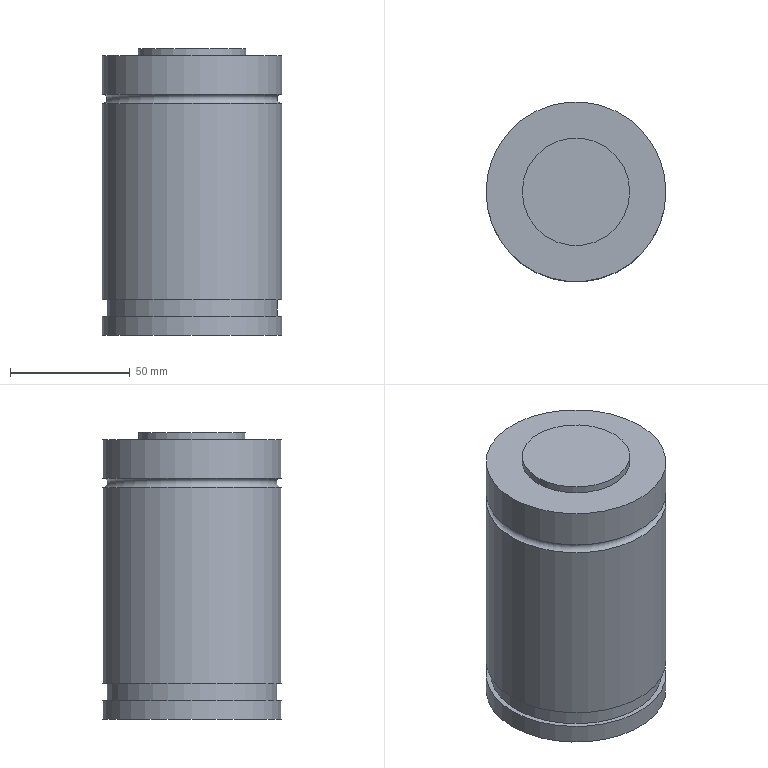Part | NX | features MAIN_BODY 2 | 1 solid | 11 faces | box 75.2 x 75.2 x 120 mm | volume 519752 mm3 | cylinder 5 | plane 5 | torus 1 | commonest cylinder face diameters 75.2 x3 45 x1 71.2 x1
STEP:
#1=CARTESIAN_POINT('',(-612.35,-310.,110.));
#2=VERTEX_POINT('',#1);
#3=CARTESIAN_POINT('',(-574.75,-310.,110.));
#4=DIRECTION('',(0.,0.,1.));
#5=DIRECTION('',(-1.,0.,0.));
#6=AXIS2_PLACEMENT_3D('',#3,#4,#5);
#7=CIRCLE('',#6,37.6);
#8=EDGE_CURVE('',#2,#2,#7,.F.);
#9=ORIENTED_EDGE('',*,*,#8,.F.);
#10=EDGE_LOOP('',(#9));
#11=FACE_BOUND('',#10,.T.);
#12=CARTESIAN_POINT('',(-612.35,-310.,192.));
#13=VERTEX_POINT('',#12);
#14=CARTESIAN_POINT('',(-574.75,-310.,192.));
#15=DIRECTION('',(0.,0.,1.));
#16=DIRECTION('',(-1.,0.,0.));
#17=AXIS2_PLACEMENT_3D('',#14,#15,#16);
#18=CIRCLE('',#17,37.6);
#19=EDGE_CURVE('',#13,#13,#18,.T.);
#20=ORIENTED_EDGE('',*,*,#19,.F.);
#21=EDGE_LOOP('',(#20));
#22=FACE_BOUND('',#21,.T.);
#23=CARTESIAN_POINT('',(-574.75,-310.,212.));
#24=DIRECTION('',(0.,0.,-1.));
#25=DIRECTION('',(-1.,0.,0.));
#26=AXIS2_PLACEMENT_3D('',#23,#24,#25);
#27=CYLINDRICAL_SURFACE('',#26,37.6);
#28=ADVANCED_FACE('',(#11,#22),#27,.T.);
#29=CARTESIAN_POINT('',(-537.15,-310.,212.));
#30=VERTEX_POINT('',#29);
#31=CARTESIAN_POINT('',(-574.75,-310.,212.));
#32=DIRECTION('',(0.,0.,-1.));
#33=DIRECTION('',(1.,0.,0.));
#34=AXIS2_PLACEMENT_3D('',#31,#32,#33);
#35=CIRCLE('',#34,37.6);
#36=EDGE_CURVE('',#30,#30,#35,.T.);
#37=ORIENTED_EDGE('',*,*,#36,.F.);
#38=EDGE_LOOP('',(#37));
#39=FACE_BOUND('',#38,.T.);
#40=CARTESIAN_POINT('',(-552.25,-310.,212.));
#41=VERTEX_POINT('',#40);
#42=CARTESIAN_POINT('',(-574.75,-310.,212.));
#43=DIRECTION('',(0.,0.,-1.));
#44=DIRECTION('',(1.,0.,0.));
#45=AXIS2_PLACEMENT_3D('',#42,#43,#44);
#46=CIRCLE('',#45,22.5);
#47=EDGE_CURVE('',#41,#41,#46,.T.);
#48=ORIENTED_EDGE('',*,*,#47,.T.);
#49=EDGE_LOOP('',(#48));
#50=FACE_BOUND('',#49,.T.);
#51=CARTESIAN_POINT('',(-574.75,-310.,212.));
#52=DIRECTION('',(0.,0.,1.));
#53=DIRECTION('',(1.,0.,0.));
#54=AXIS2_PLACEMENT_3D('',#51,#52,#53);
#55=PLANE('',#54);
#56=ADVANCED_FACE('',(#39,#50),#55,.T.);
#57=CARTESIAN_POINT('',(-612.35,-310.,196.));
#58=VERTEX_POINT('',#57);
#59=CARTESIAN_POINT('',(-574.75,-310.,196.));
#60=DIRECTION('',(0.,0.,1.));
#61=DIRECTION('',(-1.,0.,0.));
#62=AXIS2_PLACEMENT_3D('',#59,#60,#61);
#63=CIRCLE('',#62,37.6);
#64=EDGE_CURVE('',#58,#58,#63,.F.);
#65=ORIENTED_EDGE('',*,*,#64,.F.);
#66=EDGE_LOOP('',(#65));
#67=FACE_BOUND('',#66,.T.);
#68=ORIENTED_EDGE('',*,*,#36,.T.);
#69=EDGE_LOOP('',(#68));
#70=FACE_BOUND('',#69,.T.);
#71=CARTESIAN_POINT('',(-574.75,-310.,212.));
#72=DIRECTION('',(0.,0.,-1.));
#73=DIRECTION('',(-1.,0.,0.));
#74=AXIS2_PLACEMENT_3D('',#71,#72,#73);
#75=CYLINDRICAL_SURFACE('',#74,37.6);
#76=ADVANCED_FACE('',(#67,#70),#75,.T.);
#77=CARTESIAN_POINT('',(-552.25,-310.,215.));
#78=VERTEX_POINT('',#77);
#79=CARTESIAN_POINT('',(-574.75,-310.,215.));
#80=DIRECTION('',(0.,0.,-1.));
#81=DIRECTION('',(1.,0.,0.));
#82=AXIS2_PLACEMENT_3D('',#79,#80,#81);
#83=CIRCLE('',#82,22.5);
#84=EDGE_CURVE('',#78,#78,#83,.T.);
#85=ORIENTED_EDGE('',*,*,#84,.T.);
#86=EDGE_LOOP('',(#85));
#87=FACE_BOUND('',#86,.T.);
#88=ORIENTED_EDGE('',*,*,#47,.F.);
#89=EDGE_LOOP('',(#88));
#90=FACE_BOUND('',#89,.T.);
#91=CARTESIAN_POINT('',(-574.75,-310.,215.));
#92=DIRECTION('',(0.,0.,-1.));
#93=DIRECTION('',(-1.,0.,0.));
#94=AXIS2_PLACEMENT_3D('',#91,#92,#93);
#95=CYLINDRICAL_SURFACE('',#94,22.5);
#96=ADVANCED_FACE('',(#87,#90),#95,.T.);
#97=ORIENTED_EDGE('',*,*,#84,.F.);
#98=EDGE_LOOP('',(#97));
#99=FACE_BOUND('',#98,.T.);
#100=CARTESIAN_POINT('',(-574.75,-310.,215.));
#101=DIRECTION('',(0.,0.,1.));
#102=DIRECTION('',(1.,0.,0.));
#103=AXIS2_PLACEMENT_3D('',#100,#101,#102);
#104=PLANE('',#103);
#105=ADVANCED_FACE('',(#99),#104,.T.);
#106=ORIENTED_EDGE('',*,*,#64,.T.);
#107=EDGE_LOOP('',(#106));
#108=FACE_BOUND('',#107,.T.);
#109=ORIENTED_EDGE('',*,*,#19,.T.);
#110=EDGE_LOOP('',(#109));
#111=FACE_BOUND('',#110,.T.);
#112=CARTESIAN_POINT('',(-574.75,-310.,194.));
#113=DIRECTION('',(0.,0.,-1.));
#114=DIRECTION('',(-1.,0.,0.));
#115=AXIS2_PLACEMENT_3D('',#112,#113,#114);
#116=TOROIDAL_SURFACE('',#115,37.6,2.);
#117=ADVANCED_FACE('',(#108,#111),#116,.F.);
#118=CARTESIAN_POINT('',(-539.15,-310.,110.));
#119=VERTEX_POINT('',#118);
#120=CARTESIAN_POINT('',(-574.75,-310.,110.));
#121=DIRECTION('',(0.,0.,-1.));
#122=DIRECTION('',(1.,0.,0.));
#123=AXIS2_PLACEMENT_3D('',#120,#121,#122);
#124=CIRCLE('',#123,35.6);
#125=EDGE_CURVE('',#119,#119,#124,.T.);
#126=ORIENTED_EDGE('',*,*,#125,.F.);
#127=EDGE_LOOP('',(#126));
#128=FACE_BOUND('',#127,.T.);
#129=ORIENTED_EDGE('',*,*,#8,.T.);
#130=EDGE_LOOP('',(#129));
#131=FACE_BOUND('',#130,.T.);
#132=CARTESIAN_POINT('',(-574.75,-310.,110.));
#133=DIRECTION('',(0.,0.,-1.));
#134=DIRECTION('',(-1.,0.,0.));
#135=AXIS2_PLACEMENT_3D('',#132,#133,#134);
#136=PLANE('',#135);
#137=ADVANCED_FACE('',(#128,#131),#136,.T.);
#138=CARTESIAN_POINT('',(-539.15,-310.,103.));
#139=VERTEX_POINT('',#138);
#140=CARTESIAN_POINT('',(-574.75,-310.,103.));
#141=DIRECTION('',(0.,0.,-1.));
#142=DIRECTION('',(1.,0.,0.));
#143=AXIS2_PLACEMENT_3D('',#140,#141,#142);
#144=CIRCLE('',#143,35.6);
#145=EDGE_CURVE('',#139,#139,#144,.T.);
#146=ORIENTED_EDGE('',*,*,#145,.T.);
#147=EDGE_LOOP('',(#146));
#148=FACE_BOUND('',#147,.T.);
#149=CARTESIAN_POINT('',(-612.35,-310.,103.));
#150=VERTEX_POINT('',#149);
#151=CARTESIAN_POINT('',(-574.75,-310.,103.));
#152=DIRECTION('',(0.,0.,1.));
#153=DIRECTION('',(-1.,0.,0.));
#154=AXIS2_PLACEMENT_3D('',#151,#152,#153);
#155=CIRCLE('',#154,37.6);
#156=EDGE_CURVE('',#150,#150,#155,.T.);
#157=ORIENTED_EDGE('',*,*,#156,.T.);
#158=EDGE_LOOP('',(#157));
#159=FACE_BOUND('',#158,.T.);
#160=CARTESIAN_POINT('',(-574.75,-310.,103.));
#161=DIRECTION('',(0.,0.,-1.));
#162=DIRECTION('',(-1.,0.,0.));
#163=AXIS2_PLACEMENT_3D('',#160,#161,#162);
#164=PLANE('',#163);
#165=ADVANCED_FACE('',(#148,#159),#164,.F.);
#166=ORIENTED_EDGE('',*,*,#125,.T.);
#167=EDGE_LOOP('',(#166));
#168=FACE_BOUND('',#167,.T.);
#169=ORIENTED_EDGE('',*,*,#145,.F.);
#170=EDGE_LOOP('',(#169));
#171=FACE_BOUND('',#170,.T.);
#172=CARTESIAN_POINT('',(-574.75,-310.,103.));
#173=DIRECTION('',(0.,0.,1.));
#174=DIRECTION('',(1.,0.,0.));
#175=AXIS2_PLACEMENT_3D('',#172,#173,#174);
#176=CYLINDRICAL_SURFACE('',#175,35.6);
#177=ADVANCED_FACE('',(#168,#171),#176,.T.);
#178=CARTESIAN_POINT('',(-537.15,-310.,95.));
#179=VERTEX_POINT('',#178);
#180=CARTESIAN_POINT('',(-574.75,-310.,95.));
#181=DIRECTION('',(0.,0.,-1.));
#182=DIRECTION('',(1.,0.,0.));
#183=AXIS2_PLACEMENT_3D('',#180,#181,#182);
#184=CIRCLE('',#183,37.6);
#185=EDGE_CURVE('',#179,#179,#184,.T.);
#186=ORIENTED_EDGE('',*,*,#185,.T.);
#187=EDGE_LOOP('',(#186));
#188=FACE_BOUND('',#187,.T.);
#189=CARTESIAN_POINT('',(-574.75,-310.,95.));
#190=DIRECTION('',(0.,0.,1.));
#191=DIRECTION('',(1.,0.,0.));
#192=AXIS2_PLACEMENT_3D('',#189,#190,#191);
#193=PLANE('',#192);
#194=ADVANCED_FACE('',(#188),#193,.F.);
#195=ORIENTED_EDGE('',*,*,#156,.F.);
#196=EDGE_LOOP('',(#195));
#197=FACE_BOUND('',#196,.T.);
#198=ORIENTED_EDGE('',*,*,#185,.F.);
#199=EDGE_LOOP('',(#198));
#200=FACE_BOUND('',#199,.T.);
#201=CARTESIAN_POINT('',(-574.75,-310.,212.));
#202=DIRECTION('',(0.,0.,-1.));
#203=DIRECTION('',(-1.,0.,0.));
#204=AXIS2_PLACEMENT_3D('',#201,#202,#203);
#205=CYLINDRICAL_SURFACE('',#204,37.6);
#206=ADVANCED_FACE('',(#197,#200),#205,.T.);
#207=CLOSED_SHELL('',(#28,#56,#76,#96,#105,#117,#137,#165,#177,#194,#206));
#208=MANIFOLD_SOLID_BREP('',#207);
#209=(LENGTH_UNIT()NAMED_UNIT(*)SI_UNIT(.MILLI.,.METRE.));
#210=UNCERTAINTY_MEASURE_WITH_UNIT(LENGTH_MEASURE(0.00001),#209,'','');
#211=(NAMED_UNIT(*)PLANE_ANGLE_UNIT()SI_UNIT($,.RADIAN.));
#212=(NAMED_UNIT(*)SI_UNIT($,.STERADIAN.)SOLID_ANGLE_UNIT());
#213=(GEOMETRIC_REPRESENTATION_CONTEXT(3)GLOBAL_UNCERTAINTY_ASSIGNED_CONTEXT((#210))GLOBAL_UNIT_ASSIGNED_CONTEXT((#209,#211,#212))REPRESENTATION_CONTEXT('',''));
#214=ADVANCED_BREP_SHAPE_REPRESENTATION('',(#208),#213);